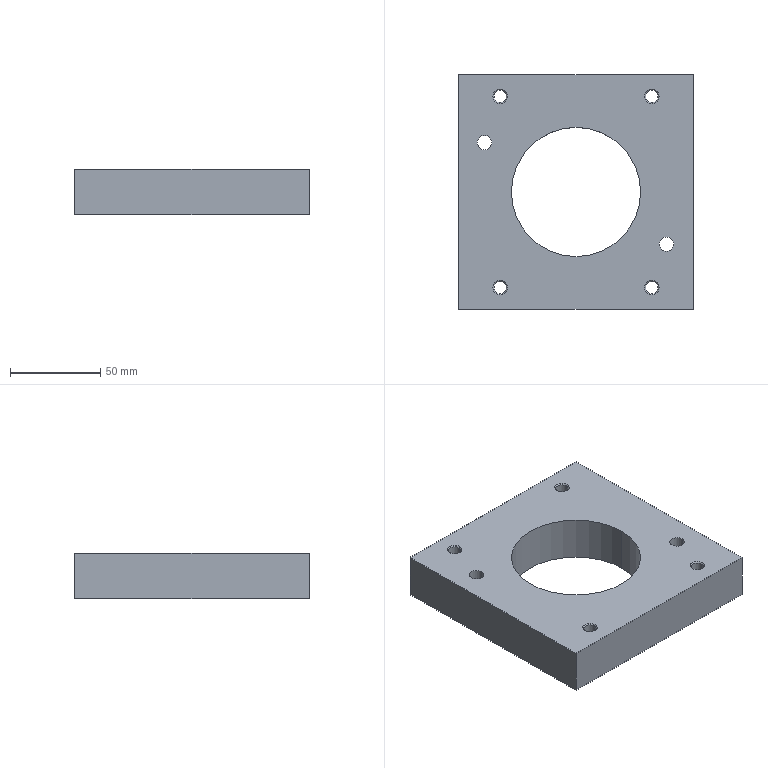Part | SolidWorks | features BaseBody 1 | 1 solid | 28 faces | box 130 x 130 x 25 mm | volume 315785 mm3 | cylinder 14 | cone 8 | plane 6 | commonest cylinder face diameters 6.806 x8 8 x4 71.56 x2
STEP:
#1=CARTESIAN_POINT('',(-131.403,-77.99,45.703));
#2=VERTEX_POINT('',#1);
#3=CARTESIAN_POINT('',(-124.597,-77.99,45.703));
#4=VERTEX_POINT('',#3);
#5=CARTESIAN_POINT('',(-128.,-77.99,45.703));
#6=DIRECTION('',(0.,0.,1.));
#7=DIRECTION('',(1.,0.,0.));
#8=AXIS2_PLACEMENT_3D('',#5,#6,#7);
#9=CIRCLE('',#8,3.403);
#10=EDGE_CURVE('',#2,#4,#9,.T.);
#11=ORIENTED_EDGE('',*,*,#10,.F.);
#12=CARTESIAN_POINT('',(-132.,-77.99,46.3));
#13=VERTEX_POINT('',#12);
#14=CARTESIAN_POINT('',(-132.,-77.99,46.3));
#15=DIRECTION('',(-0.7071,0.,0.7071));
#16=VECTOR('',#15,1000.);
#17=LINE('',#14,#16);
#18=EDGE_CURVE('',#2,#13,#17,.T.);
#19=ORIENTED_EDGE('',*,*,#18,.T.);
#20=CARTESIAN_POINT('',(-124.,-77.99,46.3));
#21=VERTEX_POINT('',#20);
#22=CARTESIAN_POINT('',(-128.,-77.99,46.3));
#23=DIRECTION('',(0.,0.,-1.));
#24=DIRECTION('',(0.7071,-0.7071,0.));
#25=AXIS2_PLACEMENT_3D('',#22,#23,#24);
#26=CIRCLE('',#25,4.);
#27=EDGE_CURVE('',#21,#13,#26,.T.);
#28=ORIENTED_EDGE('',*,*,#27,.F.);
#29=CARTESIAN_POINT('',(-124.,-77.99,46.3));
#30=DIRECTION('',(0.7071,0.,0.7071));
#31=VECTOR('',#30,1000.);
#32=LINE('',#29,#31);
#33=EDGE_CURVE('',#4,#21,#32,.T.);
#34=ORIENTED_EDGE('',*,*,#33,.F.);
#35=EDGE_LOOP('',(#11,#19,#28,#34));
#36=FACE_OUTER_BOUND('',#35,.T.);
#37=CARTESIAN_POINT('',(-128.,-77.99,46.3));
#38=DIRECTION('',(0.,0.,1.));
#39=DIRECTION('',(1.,0.,0.));
#40=AXIS2_PLACEMENT_3D('',#37,#38,#39);
#41=CONICAL_SURFACE('',#40,4.,0.7854);
#42=ADVANCED_FACE('',(#36),#41,.F.);
#43=CARTESIAN_POINT('',(-124.597,-77.99,21.3));
#44=VERTEX_POINT('',#43);
#45=CARTESIAN_POINT('',(-131.403,-77.99,21.3));
#46=VERTEX_POINT('',#45);
#47=CARTESIAN_POINT('',(-128.,-77.99,21.3));
#48=DIRECTION('',(0.,0.,-1.));
#49=DIRECTION('',(-1.,0.,0.));
#50=AXIS2_PLACEMENT_3D('',#47,#48,#49);
#51=CIRCLE('',#50,3.403);
#52=EDGE_CURVE('',#44,#46,#51,.T.);
#53=ORIENTED_EDGE('',*,*,#52,.T.);
#54=CARTESIAN_POINT('',(-131.403,-77.99,17.317));
#55=DIRECTION('',(0.,0.,1.));
#56=VECTOR('',#55,1000.);
#57=LINE('',#54,#56);
#58=EDGE_CURVE('',#46,#2,#57,.T.);
#59=ORIENTED_EDGE('',*,*,#58,.T.);
#60=ORIENTED_EDGE('',*,*,#10,.T.);
#61=CARTESIAN_POINT('',(-124.597,-77.99,17.317));
#62=DIRECTION('',(0.,0.,1.));
#63=VECTOR('',#62,1000.);
#64=LINE('',#61,#63);
#65=EDGE_CURVE('',#44,#4,#64,.T.);
#66=ORIENTED_EDGE('',*,*,#65,.F.);
#67=EDGE_LOOP('',(#53,#59,#60,#66));
#68=FACE_OUTER_BOUND('',#67,.T.);
#69=CARTESIAN_POINT('',(-128.,-77.99,17.317));
#70=DIRECTION('',(0.,0.,1.));
#71=DIRECTION('',(1.,0.,0.));
#72=AXIS2_PLACEMENT_3D('',#69,#70,#71);
#73=CYLINDRICAL_SURFACE('',#72,3.403);
#74=ADVANCED_FACE('',(#68),#73,.F.);
#75=CARTESIAN_POINT('',(-40.597,27.99,45.703));
#76=VERTEX_POINT('',#75);
#77=CARTESIAN_POINT('',(-47.403,27.99,45.703));
#78=VERTEX_POINT('',#77);
#79=CARTESIAN_POINT('',(-44.,27.99,45.703));
#80=DIRECTION('',(0.,0.,1.));
#81=DIRECTION('',(-1.,0.,0.));
#82=AXIS2_PLACEMENT_3D('',#79,#80,#81);
#83=CIRCLE('',#82,3.403);
#84=EDGE_CURVE('',#76,#78,#83,.T.);
#85=ORIENTED_EDGE('',*,*,#84,.F.);
#86=CARTESIAN_POINT('',(-40.,27.99,46.3));
#87=VERTEX_POINT('',#86);
#88=CARTESIAN_POINT('',(-40.,27.99,46.3));
#89=DIRECTION('',(0.7071,0.,0.7071));
#90=VECTOR('',#89,1000.);
#91=LINE('',#88,#90);
#92=EDGE_CURVE('',#76,#87,#91,.T.);
#93=ORIENTED_EDGE('',*,*,#92,.T.);
#94=CARTESIAN_POINT('',(-48.,27.99,46.3));
#95=VERTEX_POINT('',#94);
#96=CARTESIAN_POINT('',(-44.,27.99,46.3));
#97=DIRECTION('',(0.,0.,-1.));
#98=DIRECTION('',(-0.7071,0.7071,0.));
#99=AXIS2_PLACEMENT_3D('',#96,#97,#98);
#100=CIRCLE('',#99,4.);
#101=EDGE_CURVE('',#95,#87,#100,.T.);
#102=ORIENTED_EDGE('',*,*,#101,.F.);
#103=CARTESIAN_POINT('',(-48.,27.99,46.3));
#104=DIRECTION('',(-0.7071,0.,0.7071));
#105=VECTOR('',#104,1000.);
#106=LINE('',#103,#105);
#107=EDGE_CURVE('',#78,#95,#106,.T.);
#108=ORIENTED_EDGE('',*,*,#107,.F.);
#109=EDGE_LOOP('',(#85,#93,#102,#108));
#110=FACE_OUTER_BOUND('',#109,.T.);
#111=CARTESIAN_POINT('',(-44.,27.99,46.3));
#112=DIRECTION('',(0.,0.,1.));
#113=DIRECTION('',(-1.,0.,0.));
#114=AXIS2_PLACEMENT_3D('',#111,#112,#113);
#115=CONICAL_SURFACE('',#114,4.,0.7854);
#116=ADVANCED_FACE('',(#110),#115,.F.);
#117=CARTESIAN_POINT('',(-47.403,27.99,21.3));
#118=VERTEX_POINT('',#117);
#119=CARTESIAN_POINT('',(-40.597,27.99,21.3));
#120=VERTEX_POINT('',#119);
#121=CARTESIAN_POINT('',(-44.,27.99,21.3));
#122=DIRECTION('',(0.,0.,-1.));
#123=DIRECTION('',(-1.,0.,0.));
#124=AXIS2_PLACEMENT_3D('',#121,#122,#123);
#125=CIRCLE('',#124,3.403);
#126=EDGE_CURVE('',#118,#120,#125,.T.);
#127=ORIENTED_EDGE('',*,*,#126,.T.);
#128=CARTESIAN_POINT('',(-40.597,27.99,17.317));
#129=DIRECTION('',(0.,0.,1.));
#130=VECTOR('',#129,1000.);
#131=LINE('',#128,#130);
#132=EDGE_CURVE('',#120,#76,#131,.T.);
#133=ORIENTED_EDGE('',*,*,#132,.T.);
#134=ORIENTED_EDGE('',*,*,#84,.T.);
#135=CARTESIAN_POINT('',(-47.403,27.99,17.317));
#136=DIRECTION('',(0.,0.,1.));
#137=VECTOR('',#136,1000.);
#138=LINE('',#135,#137);
#139=EDGE_CURVE('',#118,#78,#138,.T.);
#140=ORIENTED_EDGE('',*,*,#139,.F.);
#141=EDGE_LOOP('',(#127,#133,#134,#140));
#142=FACE_OUTER_BOUND('',#141,.T.);
#143=CARTESIAN_POINT('',(-44.,27.99,17.317));
#144=DIRECTION('',(0.,0.,1.));
#145=DIRECTION('',(-1.,0.,0.));
#146=AXIS2_PLACEMENT_3D('',#143,#144,#145);
#147=CYLINDRICAL_SURFACE('',#146,3.403);
#148=ADVANCED_FACE('',(#142),#147,.F.);
#149=CARTESIAN_POINT('',(-140.678,2.312,21.3));
#150=VERTEX_POINT('',#149);
#151=CARTESIAN_POINT('',(-132.678,2.312,21.3));
#152=VERTEX_POINT('',#151);
#153=CARTESIAN_POINT('',(-136.678,2.312,21.3));
#154=DIRECTION('',(0.,0.,1.));
#155=DIRECTION('',(0.7071,0.7071,0.));
#156=AXIS2_PLACEMENT_3D('',#153,#154,#155);
#157=CIRCLE('',#156,4.);
#158=EDGE_CURVE('',#150,#152,#157,.T.);
#159=ORIENTED_EDGE('',*,*,#158,.F.);
#160=CARTESIAN_POINT('',(-140.678,2.312,46.3));
#161=VERTEX_POINT('',#160);
#162=CARTESIAN_POINT('',(-140.678,2.312,21.3));
#163=DIRECTION('',(0.,0.,1.));
#164=VECTOR('',#163,1000.);
#165=LINE('',#162,#164);
#166=EDGE_CURVE('',#150,#161,#165,.T.);
#167=ORIENTED_EDGE('',*,*,#166,.T.);
#168=CARTESIAN_POINT('',(-132.678,2.312,46.3));
#169=VERTEX_POINT('',#168);
#170=CARTESIAN_POINT('',(-136.678,2.312,46.3));
#171=DIRECTION('',(0.,0.,1.));
#172=DIRECTION('',(0.7071,0.7071,0.));
#173=AXIS2_PLACEMENT_3D('',#170,#171,#172);
#174=CIRCLE('',#173,4.);
#175=EDGE_CURVE('',#161,#169,#174,.T.);
#176=ORIENTED_EDGE('',*,*,#175,.T.);
#177=CARTESIAN_POINT('',(-132.678,2.312,21.3));
#178=DIRECTION('',(0.,0.,1.));
#179=VECTOR('',#178,1000.);
#180=LINE('',#177,#179);
#181=EDGE_CURVE('',#152,#169,#180,.T.);
#182=ORIENTED_EDGE('',*,*,#181,.F.);
#183=EDGE_LOOP('',(#159,#167,#176,#182));
#184=FACE_OUTER_BOUND('',#183,.T.);
#185=CARTESIAN_POINT('',(-136.678,2.312,21.3));
#186=DIRECTION('',(0.,0.,1.));
#187=DIRECTION('',(1.,0.,0.));
#188=AXIS2_PLACEMENT_3D('',#185,#186,#187);
#189=CYLINDRICAL_SURFACE('',#188,4.);
#190=ADVANCED_FACE('',(#184),#189,.F.);
#191=CARTESIAN_POINT('',(-39.858,-53.934,21.3));
#192=VERTEX_POINT('',#191);
#193=CARTESIAN_POINT('',(-31.858,-53.934,21.3));
#194=VERTEX_POINT('',#193);
#195=CARTESIAN_POINT('',(-35.858,-53.934,21.3));
#196=DIRECTION('',(0.,0.,1.));
#197=DIRECTION('',(0.7071,0.7071,0.));
#198=AXIS2_PLACEMENT_3D('',#195,#196,#197);
#199=CIRCLE('',#198,4.);
#200=EDGE_CURVE('',#192,#194,#199,.T.);
#201=ORIENTED_EDGE('',*,*,#200,.F.);
#202=CARTESIAN_POINT('',(-39.858,-53.934,46.3));
#203=VERTEX_POINT('',#202);
#204=CARTESIAN_POINT('',(-39.858,-53.934,21.3));
#205=DIRECTION('',(0.,0.,1.));
#206=VECTOR('',#205,1000.);
#207=LINE('',#204,#206);
#208=EDGE_CURVE('',#192,#203,#207,.T.);
#209=ORIENTED_EDGE('',*,*,#208,.T.);
#210=CARTESIAN_POINT('',(-31.858,-53.934,46.3));
#211=VERTEX_POINT('',#210);
#212=CARTESIAN_POINT('',(-35.858,-53.934,46.3));
#213=DIRECTION('',(0.,0.,1.));
#214=DIRECTION('',(0.7071,0.7071,0.));
#215=AXIS2_PLACEMENT_3D('',#212,#213,#214);
#216=CIRCLE('',#215,4.);
#217=EDGE_CURVE('',#203,#211,#216,.T.);
#218=ORIENTED_EDGE('',*,*,#217,.T.);
#219=CARTESIAN_POINT('',(-31.858,-53.934,21.3));
#220=DIRECTION('',(0.,0.,1.));
#221=VECTOR('',#220,1000.);
#222=LINE('',#219,#221);
#223=EDGE_CURVE('',#194,#211,#222,.T.);
#224=ORIENTED_EDGE('',*,*,#223,.F.);
#225=EDGE_LOOP('',(#201,#209,#218,#224));
#226=FACE_OUTER_BOUND('',#225,.T.);
#227=CARTESIAN_POINT('',(-35.858,-53.934,21.3));
#228=DIRECTION('',(0.,0.,1.));
#229=DIRECTION('',(1.,0.,0.));
#230=AXIS2_PLACEMENT_3D('',#227,#228,#229);
#231=CYLINDRICAL_SURFACE('',#230,4.);
#232=ADVANCED_FACE('',(#226),#231,.F.);
#233=CARTESIAN_POINT('',(-47.403,-77.99,45.703));
#234=VERTEX_POINT('',#233);
#235=CARTESIAN_POINT('',(-40.597,-77.99,45.703));
#236=VERTEX_POINT('',#235);
#237=CARTESIAN_POINT('',(-44.,-77.99,45.703));
#238=DIRECTION('',(0.,0.,-1.));
#239=DIRECTION('',(-1.,0.,0.));
#240=AXIS2_PLACEMENT_3D('',#237,#238,#239);
#241=CIRCLE('',#240,3.403);
#242=EDGE_CURVE('',#234,#236,#241,.T.);
#243=ORIENTED_EDGE('',*,*,#242,.T.);
#244=CARTESIAN_POINT('',(-40.,-77.99,46.3));
#245=VERTEX_POINT('',#244);
#246=CARTESIAN_POINT('',(-40.,-77.99,46.3));
#247=DIRECTION('',(0.7071,0.,0.7071));
#248=VECTOR('',#247,1000.);
#249=LINE('',#246,#248);
#250=EDGE_CURVE('',#236,#245,#249,.T.);
#251=ORIENTED_EDGE('',*,*,#250,.T.);
#252=CARTESIAN_POINT('',(-48.,-77.99,46.3));
#253=VERTEX_POINT('',#252);
#254=CARTESIAN_POINT('',(-44.,-77.99,46.3));
#255=DIRECTION('',(0.,0.,1.));
#256=DIRECTION('',(-0.7071,-0.7071,0.));
#257=AXIS2_PLACEMENT_3D('',#254,#255,#256);
#258=CIRCLE('',#257,4.);
#259=EDGE_CURVE('',#245,#253,#258,.T.);
#260=ORIENTED_EDGE('',*,*,#259,.T.);
#261=CARTESIAN_POINT('',(-48.,-77.99,46.3));
#262=DIRECTION('',(-0.7071,0.,0.7071));
#263=VECTOR('',#262,1000.);
#264=LINE('',#261,#263);
#265=EDGE_CURVE('',#234,#253,#264,.T.);
#266=ORIENTED_EDGE('',*,*,#265,.F.);
#267=EDGE_LOOP('',(#243,#251,#260,#266));
#268=FACE_OUTER_BOUND('',#267,.T.);
#269=CARTESIAN_POINT('',(-44.,-77.99,46.3));
#270=DIRECTION('',(0.,0.,1.));
#271=DIRECTION('',(-1.,0.,0.));
#272=AXIS2_PLACEMENT_3D('',#269,#270,#271);
#273=CONICAL_SURFACE('',#272,4.,0.7854);
#274=ADVANCED_FACE('',(#268),#273,.F.);
#275=CARTESIAN_POINT('',(-47.403,-77.99,21.3));
#276=VERTEX_POINT('',#275);
#277=CARTESIAN_POINT('',(-40.597,-77.99,21.3));
#278=VERTEX_POINT('',#277);
#279=CARTESIAN_POINT('',(-44.,-77.99,21.3));
#280=DIRECTION('',(0.,0.,-1.));
#281=DIRECTION('',(-1.,0.,0.));
#282=AXIS2_PLACEMENT_3D('',#279,#280,#281);
#283=CIRCLE('',#282,3.403);
#284=EDGE_CURVE('',#276,#278,#283,.T.);
#285=ORIENTED_EDGE('',*,*,#284,.T.);
#286=CARTESIAN_POINT('',(-40.597,-77.99,17.317));
#287=DIRECTION('',(0.,0.,1.));
#288=VECTOR('',#287,1000.);
#289=LINE('',#286,#288);
#290=EDGE_CURVE('',#278,#236,#289,.T.);
#291=ORIENTED_EDGE('',*,*,#290,.T.);
#292=ORIENTED_EDGE('',*,*,#242,.F.);
#293=CARTESIAN_POINT('',(-47.403,-77.99,17.317));
#294=DIRECTION('',(0.,0.,1.));
#295=VECTOR('',#294,1000.);
#296=LINE('',#293,#295);
#297=EDGE_CURVE('',#276,#234,#296,.T.);
#298=ORIENTED_EDGE('',*,*,#297,.F.);
#299=EDGE_LOOP('',(#285,#291,#292,#298));
#300=FACE_OUTER_BOUND('',#299,.T.);
#301=CARTESIAN_POINT('',(-44.,-77.99,17.317));
#302=DIRECTION('',(0.,0.,1.));
#303=DIRECTION('',(-1.,0.,0.));
#304=AXIS2_PLACEMENT_3D('',#301,#302,#303);
#305=CYLINDRICAL_SURFACE('',#304,3.403);
#306=ADVANCED_FACE('',(#300),#305,.F.);
#307=CARTESIAN_POINT('',(-124.597,27.99,45.703));
#308=VERTEX_POINT('',#307);
#309=CARTESIAN_POINT('',(-131.403,27.99,45.703));
#310=VERTEX_POINT('',#309);
#311=CARTESIAN_POINT('',(-128.,27.99,45.703));
#312=DIRECTION('',(0.,0.,-1.));
#313=DIRECTION('',(1.,0.,0.));
#314=AXIS2_PLACEMENT_3D('',#311,#312,#313);
#315=CIRCLE('',#314,3.403);
#316=EDGE_CURVE('',#308,#310,#315,.T.);
#317=ORIENTED_EDGE('',*,*,#316,.T.);
#318=CARTESIAN_POINT('',(-132.,27.99,46.3));
#319=VERTEX_POINT('',#318);
#320=CARTESIAN_POINT('',(-132.,27.99,46.3));
#321=DIRECTION('',(-0.7071,0.,0.7071));
#322=VECTOR('',#321,1000.);
#323=LINE('',#320,#322);
#324=EDGE_CURVE('',#310,#319,#323,.T.);
#325=ORIENTED_EDGE('',*,*,#324,.T.);
#326=CARTESIAN_POINT('',(-124.,27.99,46.3));
#327=VERTEX_POINT('',#326);
#328=CARTESIAN_POINT('',(-128.,27.99,46.3));
#329=DIRECTION('',(0.,0.,1.));
#330=DIRECTION('',(0.7071,0.7071,0.));
#331=AXIS2_PLACEMENT_3D('',#328,#329,#330);
#332=CIRCLE('',#331,4.);
#333=EDGE_CURVE('',#319,#327,#332,.T.);
#334=ORIENTED_EDGE('',*,*,#333,.T.);
#335=CARTESIAN_POINT('',(-124.,27.99,46.3));
#336=DIRECTION('',(0.7071,0.,0.7071));
#337=VECTOR('',#336,1000.);
#338=LINE('',#335,#337);
#339=EDGE_CURVE('',#308,#327,#338,.T.);
#340=ORIENTED_EDGE('',*,*,#339,.F.);
#341=EDGE_LOOP('',(#317,#325,#334,#340));
#342=FACE_OUTER_BOUND('',#341,.T.);
#343=CARTESIAN_POINT('',(-128.,27.99,46.3));
#344=DIRECTION('',(0.,0.,1.));
#345=DIRECTION('',(1.,0.,0.));
#346=AXIS2_PLACEMENT_3D('',#343,#344,#345);
#347=CONICAL_SURFACE('',#346,4.,0.7854);
#348=ADVANCED_FACE('',(#342),#347,.F.);
#349=CARTESIAN_POINT('',(-124.597,27.99,21.3));
#350=VERTEX_POINT('',#349);
#351=CARTESIAN_POINT('',(-131.403,27.99,21.3));
#352=VERTEX_POINT('',#351);
#353=CARTESIAN_POINT('',(-128.,27.99,21.3));
#354=DIRECTION('',(0.,0.,-1.));
#355=DIRECTION('',(-1.,0.,0.));
#356=AXIS2_PLACEMENT_3D('',#353,#354,#355);
#357=CIRCLE('',#356,3.403);
#358=EDGE_CURVE('',#350,#352,#357,.T.);
#359=ORIENTED_EDGE('',*,*,#358,.T.);
#360=CARTESIAN_POINT('',(-131.403,27.99,17.317));
#361=DIRECTION('',(0.,0.,1.));
#362=VECTOR('',#361,1000.);
#363=LINE('',#360,#362);
#364=EDGE_CURVE('',#352,#310,#363,.T.);
#365=ORIENTED_EDGE('',*,*,#364,.T.);
#366=ORIENTED_EDGE('',*,*,#316,.F.);
#367=CARTESIAN_POINT('',(-124.597,27.99,17.317));
#368=DIRECTION('',(0.,0.,1.));
#369=VECTOR('',#368,1000.);
#370=LINE('',#367,#369);
#371=EDGE_CURVE('',#350,#308,#370,.T.);
#372=ORIENTED_EDGE('',*,*,#371,.F.);
#373=EDGE_LOOP('',(#359,#365,#366,#372));
#374=FACE_OUTER_BOUND('',#373,.T.);
#375=CARTESIAN_POINT('',(-128.,27.99,17.317));
#376=DIRECTION('',(0.,0.,1.));
#377=DIRECTION('',(1.,0.,0.));
#378=AXIS2_PLACEMENT_3D('',#375,#376,#377);
#379=CYLINDRICAL_SURFACE('',#378,3.403);
#380=ADVANCED_FACE('',(#374),#379,.F.);
#381=CARTESIAN_POINT('',(-50.22,-25.,46.3));
#382=VERTEX_POINT('',#381);
#383=CARTESIAN_POINT('',(-121.78,-25.,46.3));
#384=VERTEX_POINT('',#383);
#385=CARTESIAN_POINT('',(-86.,-25.,46.3));
#386=DIRECTION('',(0.,0.,-1.));
#387=DIRECTION('',(-1.,0.,0.));
#388=AXIS2_PLACEMENT_3D('',#385,#386,#387);
#389=CIRCLE('',#388,35.78);
#390=EDGE_CURVE('',#382,#384,#389,.T.);
#391=ORIENTED_EDGE('',*,*,#390,.F.);
#392=CARTESIAN_POINT('',(-50.22,-25.,21.3));
#393=VERTEX_POINT('',#392);
#394=CARTESIAN_POINT('',(-50.22,-25.,21.3));
#395=DIRECTION('',(0.,0.,-1.));
#396=VECTOR('',#395,1000.);
#397=LINE('',#394,#396);
#398=EDGE_CURVE('',#382,#393,#397,.T.);
#399=ORIENTED_EDGE('',*,*,#398,.T.);
#400=CARTESIAN_POINT('',(-121.78,-25.,21.3));
#401=VERTEX_POINT('',#400);
#402=CARTESIAN_POINT('',(-86.,-25.,21.3));
#403=DIRECTION('',(0.,0.,-1.));
#404=DIRECTION('',(-1.,0.,0.));
#405=AXIS2_PLACEMENT_3D('',#402,#403,#404);
#406=CIRCLE('',#405,35.78);
#407=EDGE_CURVE('',#393,#401,#406,.T.);
#408=ORIENTED_EDGE('',*,*,#407,.T.);
#409=CARTESIAN_POINT('',(-121.78,-25.,21.3));
#410=DIRECTION('',(0.,0.,-1.));
#411=VECTOR('',#410,1000.);
#412=LINE('',#409,#411);
#413=EDGE_CURVE('',#384,#401,#412,.T.);
#414=ORIENTED_EDGE('',*,*,#413,.F.);
#415=EDGE_LOOP('',(#391,#399,#408,#414));
#416=FACE_OUTER_BOUND('',#415,.T.);
#417=CARTESIAN_POINT('',(-86.,-25.,21.3));
#418=DIRECTION('',(0.,0.,-1.));
#419=DIRECTION('',(-1.,0.,0.));
#420=AXIS2_PLACEMENT_3D('',#417,#418,#419);
#421=CYLINDRICAL_SURFACE('',#420,35.78);
#422=ADVANCED_FACE('',(#416),#421,.F.);
#423=CARTESIAN_POINT('',(-21.,40.,21.3));
#424=VERTEX_POINT('',#423);
#425=CARTESIAN_POINT('',(-21.,40.,46.3));
#426=VERTEX_POINT('',#425);
#427=CARTESIAN_POINT('',(-21.,40.,21.3));
#428=DIRECTION('',(0.,0.,1.));
#429=VECTOR('',#428,1000.);
#430=LINE('',#427,#429);
#431=EDGE_CURVE('',#424,#426,#430,.T.);
#432=ORIENTED_EDGE('',*,*,#431,.F.);
#433=CARTESIAN_POINT('',(-151.,40.,21.3));
#434=VERTEX_POINT('',#433);
#435=CARTESIAN_POINT('',(-86.,40.,21.3));
#436=DIRECTION('',(-1.,0.,0.));
#437=VECTOR('',#436,1000.);
#438=LINE('',#435,#437);
#439=EDGE_CURVE('',#424,#434,#438,.T.);
#440=ORIENTED_EDGE('',*,*,#439,.T.);
#441=CARTESIAN_POINT('',(-151.,40.,46.3));
#442=VERTEX_POINT('',#441);
#443=CARTESIAN_POINT('',(-151.,40.,21.3));
#444=DIRECTION('',(0.,0.,1.));
#445=VECTOR('',#444,1000.);
#446=LINE('',#443,#445);
#447=EDGE_CURVE('',#434,#442,#446,.T.);
#448=ORIENTED_EDGE('',*,*,#447,.T.);
#449=CARTESIAN_POINT('',(-86.,40.,46.3));
#450=DIRECTION('',(-1.,0.,0.));
#451=VECTOR('',#450,1000.);
#452=LINE('',#449,#451);
#453=EDGE_CURVE('',#426,#442,#452,.T.);
#454=ORIENTED_EDGE('',*,*,#453,.F.);
#455=EDGE_LOOP('',(#432,#440,#448,#454));
#456=FACE_OUTER_BOUND('',#455,.T.);
#457=CARTESIAN_POINT('',(-86.,40.,21.3));
#458=DIRECTION('',(0.,-1.,0.));
#459=DIRECTION('',(-1.,0.,0.));
#460=AXIS2_PLACEMENT_3D('',#457,#458,#459);
#461=PLANE('',#460);
#462=ADVANCED_FACE('',(#456),#461,.F.);
#463=ORIENTED_EDGE('',*,*,#447,.F.);
#464=CARTESIAN_POINT('',(-151.,-90.,21.3));
#465=VERTEX_POINT('',#464);
#466=CARTESIAN_POINT('',(-151.,-25.,21.3));
#467=DIRECTION('',(0.,-1.,0.));
#468=VECTOR('',#467,1000.);
#469=LINE('',#466,#468);
#470=EDGE_CURVE('',#434,#465,#469,.T.);
#471=ORIENTED_EDGE('',*,*,#470,.T.);
#472=CARTESIAN_POINT('',(-151.,-90.,46.3));
#473=VERTEX_POINT('',#472);
#474=CARTESIAN_POINT('',(-151.,-90.,21.3));
#475=DIRECTION('',(0.,0.,1.));
#476=VECTOR('',#475,1000.);
#477=LINE('',#474,#476);
#478=EDGE_CURVE('',#465,#473,#477,.T.);
#479=ORIENTED_EDGE('',*,*,#478,.T.);
#480=CARTESIAN_POINT('',(-151.,-25.,46.3));
#481=DIRECTION('',(0.,-1.,0.));
#482=VECTOR('',#481,1000.);
#483=LINE('',#480,#482);
#484=EDGE_CURVE('',#442,#473,#483,.T.);
#485=ORIENTED_EDGE('',*,*,#484,.F.);
#486=EDGE_LOOP('',(#463,#471,#479,#485));
#487=FACE_OUTER_BOUND('',#486,.T.);
#488=CARTESIAN_POINT('',(-151.,-25.,21.3));
#489=DIRECTION('',(1.,0.,0.));
#490=DIRECTION('',(0.,-1.,0.));
#491=AXIS2_PLACEMENT_3D('',#488,#489,#490);
#492=PLANE('',#491);
#493=ADVANCED_FACE('',(#487),#492,.F.);
#494=ORIENTED_EDGE('',*,*,#478,.F.);
#495=CARTESIAN_POINT('',(-21.,-90.,21.3));
#496=VERTEX_POINT('',#495);
#497=CARTESIAN_POINT('',(-86.,-90.,21.3));
#498=DIRECTION('',(1.,0.,0.));
#499=VECTOR('',#498,1000.);
#500=LINE('',#497,#499);
#501=EDGE_CURVE('',#465,#496,#500,.T.);
#502=ORIENTED_EDGE('',*,*,#501,.T.);
#503=CARTESIAN_POINT('',(-21.,-90.,46.3));
#504=VERTEX_POINT('',#503);
#505=CARTESIAN_POINT('',(-21.,-90.,21.3));
#506=DIRECTION('',(0.,0.,1.));
#507=VECTOR('',#506,1000.);
#508=LINE('',#505,#507);
#509=EDGE_CURVE('',#496,#504,#508,.T.);
#510=ORIENTED_EDGE('',*,*,#509,.T.);
#511=CARTESIAN_POINT('',(-86.,-90.,46.3));
#512=DIRECTION('',(1.,0.,0.));
#513=VECTOR('',#512,1000.);
#514=LINE('',#511,#513);
#515=EDGE_CURVE('',#473,#504,#514,.T.);
#516=ORIENTED_EDGE('',*,*,#515,.F.);
#517=EDGE_LOOP('',(#494,#502,#510,#516));
#518=FACE_OUTER_BOUND('',#517,.T.);
#519=CARTESIAN_POINT('',(-86.,-90.,21.3));
#520=DIRECTION('',(0.,1.,0.));
#521=DIRECTION('',(1.,0.,0.));
#522=AXIS2_PLACEMENT_3D('',#519,#520,#521);
#523=PLANE('',#522);
#524=ADVANCED_FACE('',(#518),#523,.F.);
#525=ORIENTED_EDGE('',*,*,#398,.F.);
#526=CARTESIAN_POINT('',(-86.,-25.,46.3));
#527=DIRECTION('',(0.,0.,-1.));
#528=DIRECTION('',(-1.,0.,0.));
#529=AXIS2_PLACEMENT_3D('',#526,#527,#528);
#530=CIRCLE('',#529,35.78);
#531=EDGE_CURVE('',#384,#382,#530,.T.);
#532=ORIENTED_EDGE('',*,*,#531,.F.);
#533=ORIENTED_EDGE('',*,*,#413,.T.);
#534=CARTESIAN_POINT('',(-86.,-25.,21.3));
#535=DIRECTION('',(0.,0.,-1.));
#536=DIRECTION('',(-1.,0.,0.));
#537=AXIS2_PLACEMENT_3D('',#534,#535,#536);
#538=CIRCLE('',#537,35.78);
#539=EDGE_CURVE('',#401,#393,#538,.T.);
#540=ORIENTED_EDGE('',*,*,#539,.T.);
#541=EDGE_LOOP('',(#525,#532,#533,#540));
#542=FACE_OUTER_BOUND('',#541,.T.);
#543=CARTESIAN_POINT('',(-86.,-25.,21.3));
#544=DIRECTION('',(0.,0.,-1.));
#545=DIRECTION('',(-1.,0.,0.));
#546=AXIS2_PLACEMENT_3D('',#543,#544,#545);
#547=CYLINDRICAL_SURFACE('',#546,35.78);
#548=ADVANCED_FACE('',(#542),#547,.F.);
#549=CARTESIAN_POINT('',(-21.,-25.,21.3));
#550=DIRECTION('',(0.,1.,0.));
#551=VECTOR('',#550,1000.);
#552=LINE('',#549,#551);
#553=EDGE_CURVE('',#496,#424,#552,.T.);
#554=ORIENTED_EDGE('',*,*,#553,.T.);
#555=ORIENTED_EDGE('',*,*,#431,.T.);
#556=CARTESIAN_POINT('',(-21.,-25.,46.3));
#557=DIRECTION('',(0.,1.,0.));
#558=VECTOR('',#557,1000.);
#559=LINE('',#556,#558);
#560=EDGE_CURVE('',#504,#426,#559,.T.);
#561=ORIENTED_EDGE('',*,*,#560,.F.);
#562=ORIENTED_EDGE('',*,*,#509,.F.);
#563=EDGE_LOOP('',(#554,#555,#561,#562));
#564=FACE_OUTER_BOUND('',#563,.T.);
#565=CARTESIAN_POINT('',(-21.,-25.,21.3));
#566=DIRECTION('',(-1.,0.,0.));
#567=DIRECTION('',(0.,1.,0.));
#568=AXIS2_PLACEMENT_3D('',#565,#566,#567);
#569=PLANE('',#568);
#570=ADVANCED_FACE('',(#564),#569,.F.);
#571=ORIENTED_EDGE('',*,*,#27,.T.);
#572=CARTESIAN_POINT('',(-128.,-77.99,46.3));
#573=DIRECTION('',(0.,0.,-1.));
#574=DIRECTION('',(0.7071,-0.7071,0.));
#575=AXIS2_PLACEMENT_3D('',#572,#573,#574);
#576=CIRCLE('',#575,4.);
#577=EDGE_CURVE('',#13,#21,#576,.T.);
#578=ORIENTED_EDGE('',*,*,#577,.T.);
#579=EDGE_LOOP('',(#571,#578));
#580=FACE_BOUND('',#579,.T.);
#581=ORIENTED_EDGE('',*,*,#101,.T.);
#582=CARTESIAN_POINT('',(-44.,27.99,46.3));
#583=DIRECTION('',(0.,0.,-1.));
#584=DIRECTION('',(-0.7071,0.7071,0.));
#585=AXIS2_PLACEMENT_3D('',#582,#583,#584);
#586=CIRCLE('',#585,4.);
#587=EDGE_CURVE('',#87,#95,#586,.T.);
#588=ORIENTED_EDGE('',*,*,#587,.T.);
#589=EDGE_LOOP('',(#581,#588));
#590=FACE_BOUND('',#589,.T.);
#591=CARTESIAN_POINT('',(-136.678,2.312,46.3));
#592=DIRECTION('',(0.,0.,1.));
#593=DIRECTION('',(0.7071,0.7071,0.));
#594=AXIS2_PLACEMENT_3D('',#591,#592,#593);
#595=CIRCLE('',#594,4.);
#596=EDGE_CURVE('',#169,#161,#595,.T.);
#597=ORIENTED_EDGE('',*,*,#596,.F.);
#598=ORIENTED_EDGE('',*,*,#175,.F.);
#599=EDGE_LOOP('',(#597,#598));
#600=FACE_BOUND('',#599,.T.);
#601=CARTESIAN_POINT('',(-35.858,-53.934,46.3));
#602=DIRECTION('',(0.,0.,1.));
#603=DIRECTION('',(0.7071,0.7071,0.));
#604=AXIS2_PLACEMENT_3D('',#601,#602,#603);
#605=CIRCLE('',#604,4.);
#606=EDGE_CURVE('',#211,#203,#605,.T.);
#607=ORIENTED_EDGE('',*,*,#606,.F.);
#608=ORIENTED_EDGE('',*,*,#217,.F.);
#609=EDGE_LOOP('',(#607,#608));
#610=FACE_BOUND('',#609,.T.);
#611=CARTESIAN_POINT('',(-44.,-77.99,46.3));
#612=DIRECTION('',(0.,0.,1.));
#613=DIRECTION('',(-0.7071,-0.7071,0.));
#614=AXIS2_PLACEMENT_3D('',#611,#612,#613);
#615=CIRCLE('',#614,4.);
#616=EDGE_CURVE('',#253,#245,#615,.T.);
#617=ORIENTED_EDGE('',*,*,#616,.F.);
#618=ORIENTED_EDGE('',*,*,#259,.F.);
#619=EDGE_LOOP('',(#617,#618));
#620=FACE_BOUND('',#619,.T.);
#621=CARTESIAN_POINT('',(-128.,27.99,46.3));
#622=DIRECTION('',(0.,0.,1.));
#623=DIRECTION('',(0.7071,0.7071,0.));
#624=AXIS2_PLACEMENT_3D('',#621,#622,#623);
#625=CIRCLE('',#624,4.);
#626=EDGE_CURVE('',#327,#319,#625,.T.);
#627=ORIENTED_EDGE('',*,*,#626,.F.);
#628=ORIENTED_EDGE('',*,*,#333,.F.);
#629=EDGE_LOOP('',(#627,#628));
#630=FACE_BOUND('',#629,.T.);
#631=ORIENTED_EDGE('',*,*,#531,.T.);
#632=ORIENTED_EDGE('',*,*,#390,.T.);
#633=EDGE_LOOP('',(#631,#632));
#634=FACE_BOUND('',#633,.T.);
#635=ORIENTED_EDGE('',*,*,#515,.T.);
#636=ORIENTED_EDGE('',*,*,#560,.T.);
#637=ORIENTED_EDGE('',*,*,#453,.T.);
#638=ORIENTED_EDGE('',*,*,#484,.T.);
#639=EDGE_LOOP('',(#635,#636,#637,#638));
#640=FACE_OUTER_BOUND('',#639,.T.);
#641=CARTESIAN_POINT('',(-86.,-25.,46.3));
#642=DIRECTION('',(0.,0.,-1.));
#643=DIRECTION('',(-1.,0.,0.));
#644=AXIS2_PLACEMENT_3D('',#641,#642,#643);
#645=PLANE('',#644);
#646=ADVANCED_FACE('',(#580,#590,#600,#610,#620,#630,#634,#640),#645,.F.);
#647=ORIENTED_EDGE('',*,*,#52,.F.);
#648=CARTESIAN_POINT('',(-128.,-77.99,21.3));
#649=DIRECTION('',(0.,0.,-1.));
#650=DIRECTION('',(-1.,0.,0.));
#651=AXIS2_PLACEMENT_3D('',#648,#649,#650);
#652=CIRCLE('',#651,3.403);
#653=EDGE_CURVE('',#46,#44,#652,.T.);
#654=ORIENTED_EDGE('',*,*,#653,.F.);
#655=EDGE_LOOP('',(#647,#654));
#656=FACE_BOUND('',#655,.T.);
#657=ORIENTED_EDGE('',*,*,#126,.F.);
#658=CARTESIAN_POINT('',(-44.,27.99,21.3));
#659=DIRECTION('',(0.,0.,-1.));
#660=DIRECTION('',(-1.,0.,0.));
#661=AXIS2_PLACEMENT_3D('',#658,#659,#660);
#662=CIRCLE('',#661,3.403);
#663=EDGE_CURVE('',#120,#118,#662,.T.);
#664=ORIENTED_EDGE('',*,*,#663,.F.);
#665=EDGE_LOOP('',(#657,#664));
#666=FACE_BOUND('',#665,.T.);
#667=CARTESIAN_POINT('',(-136.678,2.312,21.3));
#668=DIRECTION('',(0.,0.,1.));
#669=DIRECTION('',(0.7071,0.7071,0.));
#670=AXIS2_PLACEMENT_3D('',#667,#668,#669);
#671=CIRCLE('',#670,4.);
#672=EDGE_CURVE('',#152,#150,#671,.T.);
#673=ORIENTED_EDGE('',*,*,#672,.T.);
#674=ORIENTED_EDGE('',*,*,#158,.T.);
#675=EDGE_LOOP('',(#673,#674));
#676=FACE_BOUND('',#675,.T.);
#677=CARTESIAN_POINT('',(-35.858,-53.934,21.3));
#678=DIRECTION('',(0.,0.,1.));
#679=DIRECTION('',(0.7071,0.7071,0.));
#680=AXIS2_PLACEMENT_3D('',#677,#678,#679);
#681=CIRCLE('',#680,4.);
#682=EDGE_CURVE('',#194,#192,#681,.T.);
#683=ORIENTED_EDGE('',*,*,#682,.T.);
#684=ORIENTED_EDGE('',*,*,#200,.T.);
#685=EDGE_LOOP('',(#683,#684));
#686=FACE_BOUND('',#685,.T.);
#687=ORIENTED_EDGE('',*,*,#284,.F.);
#688=CARTESIAN_POINT('',(-44.,-77.99,21.3));
#689=DIRECTION('',(0.,0.,-1.));
#690=DIRECTION('',(-1.,0.,0.));
#691=AXIS2_PLACEMENT_3D('',#688,#689,#690);
#692=CIRCLE('',#691,3.403);
#693=EDGE_CURVE('',#278,#276,#692,.T.);
#694=ORIENTED_EDGE('',*,*,#693,.F.);
#695=EDGE_LOOP('',(#687,#694));
#696=FACE_BOUND('',#695,.T.);
#697=ORIENTED_EDGE('',*,*,#358,.F.);
#698=CARTESIAN_POINT('',(-128.,27.99,21.3));
#699=DIRECTION('',(0.,0.,-1.));
#700=DIRECTION('',(-1.,0.,0.));
#701=AXIS2_PLACEMENT_3D('',#698,#699,#700);
#702=CIRCLE('',#701,3.403);
#703=EDGE_CURVE('',#352,#350,#702,.T.);
#704=ORIENTED_EDGE('',*,*,#703,.F.);
#705=EDGE_LOOP('',(#697,#704));
#706=FACE_BOUND('',#705,.T.);
#707=ORIENTED_EDGE('',*,*,#539,.F.);
#708=ORIENTED_EDGE('',*,*,#407,.F.);
#709=EDGE_LOOP('',(#707,#708));
#710=FACE_BOUND('',#709,.T.);
#711=ORIENTED_EDGE('',*,*,#501,.F.);
#712=ORIENTED_EDGE('',*,*,#470,.F.);
#713=ORIENTED_EDGE('',*,*,#439,.F.);
#714=ORIENTED_EDGE('',*,*,#553,.F.);
#715=EDGE_LOOP('',(#711,#712,#713,#714));
#716=FACE_OUTER_BOUND('',#715,.T.);
#717=CARTESIAN_POINT('',(-86.,-25.,21.3));
#718=DIRECTION('',(0.,0.,-1.));
#719=DIRECTION('',(-1.,0.,0.));
#720=AXIS2_PLACEMENT_3D('',#717,#718,#719);
#721=PLANE('',#720);
#722=ADVANCED_FACE('',(#656,#666,#676,#686,#696,#706,#710,#716),#721,.T.);
#723=ORIENTED_EDGE('',*,*,#364,.F.);
#724=ORIENTED_EDGE('',*,*,#703,.T.);
#725=ORIENTED_EDGE('',*,*,#371,.T.);
#726=CARTESIAN_POINT('',(-128.,27.99,45.703));
#727=DIRECTION('',(0.,0.,-1.));
#728=DIRECTION('',(1.,0.,0.));
#729=AXIS2_PLACEMENT_3D('',#726,#727,#728);
#730=CIRCLE('',#729,3.403);
#731=EDGE_CURVE('',#310,#308,#730,.T.);
#732=ORIENTED_EDGE('',*,*,#731,.F.);
#733=EDGE_LOOP('',(#723,#724,#725,#732));
#734=FACE_OUTER_BOUND('',#733,.T.);
#735=CARTESIAN_POINT('',(-128.,27.99,17.317));
#736=DIRECTION('',(0.,0.,1.));
#737=DIRECTION('',(1.,0.,0.));
#738=AXIS2_PLACEMENT_3D('',#735,#736,#737);
#739=CYLINDRICAL_SURFACE('',#738,3.403);
#740=ADVANCED_FACE('',(#734),#739,.F.);
#741=ORIENTED_EDGE('',*,*,#324,.F.);
#742=ORIENTED_EDGE('',*,*,#731,.T.);
#743=ORIENTED_EDGE('',*,*,#339,.T.);
#744=ORIENTED_EDGE('',*,*,#626,.T.);
#745=EDGE_LOOP('',(#741,#742,#743,#744));
#746=FACE_OUTER_BOUND('',#745,.T.);
#747=CARTESIAN_POINT('',(-128.,27.99,46.3));
#748=DIRECTION('',(0.,0.,1.));
#749=DIRECTION('',(1.,0.,0.));
#750=AXIS2_PLACEMENT_3D('',#747,#748,#749);
#751=CONICAL_SURFACE('',#750,4.,0.7854);
#752=ADVANCED_FACE('',(#746),#751,.F.);
#753=ORIENTED_EDGE('',*,*,#290,.F.);
#754=ORIENTED_EDGE('',*,*,#693,.T.);
#755=ORIENTED_EDGE('',*,*,#297,.T.);
#756=CARTESIAN_POINT('',(-44.,-77.99,45.703));
#757=DIRECTION('',(0.,0.,-1.));
#758=DIRECTION('',(-1.,0.,0.));
#759=AXIS2_PLACEMENT_3D('',#756,#757,#758);
#760=CIRCLE('',#759,3.403);
#761=EDGE_CURVE('',#236,#234,#760,.T.);
#762=ORIENTED_EDGE('',*,*,#761,.F.);
#763=EDGE_LOOP('',(#753,#754,#755,#762));
#764=FACE_OUTER_BOUND('',#763,.T.);
#765=CARTESIAN_POINT('',(-44.,-77.99,17.317));
#766=DIRECTION('',(0.,0.,1.));
#767=DIRECTION('',(-1.,0.,0.));
#768=AXIS2_PLACEMENT_3D('',#765,#766,#767);
#769=CYLINDRICAL_SURFACE('',#768,3.403);
#770=ADVANCED_FACE('',(#764),#769,.F.);
#771=ORIENTED_EDGE('',*,*,#250,.F.);
#772=ORIENTED_EDGE('',*,*,#761,.T.);
#773=ORIENTED_EDGE('',*,*,#265,.T.);
#774=ORIENTED_EDGE('',*,*,#616,.T.);
#775=EDGE_LOOP('',(#771,#772,#773,#774));
#776=FACE_OUTER_BOUND('',#775,.T.);
#777=CARTESIAN_POINT('',(-44.,-77.99,46.3));
#778=DIRECTION('',(0.,0.,1.));
#779=DIRECTION('',(-1.,0.,0.));
#780=AXIS2_PLACEMENT_3D('',#777,#778,#779);
#781=CONICAL_SURFACE('',#780,4.,0.7854);
#782=ADVANCED_FACE('',(#776),#781,.F.);
#783=ORIENTED_EDGE('',*,*,#208,.F.);
#784=ORIENTED_EDGE('',*,*,#682,.F.);
#785=ORIENTED_EDGE('',*,*,#223,.T.);
#786=ORIENTED_EDGE('',*,*,#606,.T.);
#787=EDGE_LOOP('',(#783,#784,#785,#786));
#788=FACE_OUTER_BOUND('',#787,.T.);
#789=CARTESIAN_POINT('',(-35.858,-53.934,21.3));
#790=DIRECTION('',(0.,0.,1.));
#791=DIRECTION('',(1.,0.,0.));
#792=AXIS2_PLACEMENT_3D('',#789,#790,#791);
#793=CYLINDRICAL_SURFACE('',#792,4.);
#794=ADVANCED_FACE('',(#788),#793,.F.);
#795=ORIENTED_EDGE('',*,*,#166,.F.);
#796=ORIENTED_EDGE('',*,*,#672,.F.);
#797=ORIENTED_EDGE('',*,*,#181,.T.);
#798=ORIENTED_EDGE('',*,*,#596,.T.);
#799=EDGE_LOOP('',(#795,#796,#797,#798));
#800=FACE_OUTER_BOUND('',#799,.T.);
#801=CARTESIAN_POINT('',(-136.678,2.312,21.3));
#802=DIRECTION('',(0.,0.,1.));
#803=DIRECTION('',(1.,0.,0.));
#804=AXIS2_PLACEMENT_3D('',#801,#802,#803);
#805=CYLINDRICAL_SURFACE('',#804,4.);
#806=ADVANCED_FACE('',(#800),#805,.F.);
#807=ORIENTED_EDGE('',*,*,#132,.F.);
#808=ORIENTED_EDGE('',*,*,#663,.T.);
#809=ORIENTED_EDGE('',*,*,#139,.T.);
#810=CARTESIAN_POINT('',(-44.,27.99,45.703));
#811=DIRECTION('',(0.,0.,1.));
#812=DIRECTION('',(-1.,0.,0.));
#813=AXIS2_PLACEMENT_3D('',#810,#811,#812);
#814=CIRCLE('',#813,3.403);
#815=EDGE_CURVE('',#78,#76,#814,.T.);
#816=ORIENTED_EDGE('',*,*,#815,.T.);
#817=EDGE_LOOP('',(#807,#808,#809,#816));
#818=FACE_OUTER_BOUND('',#817,.T.);
#819=CARTESIAN_POINT('',(-44.,27.99,17.317));
#820=DIRECTION('',(0.,0.,1.));
#821=DIRECTION('',(-1.,0.,0.));
#822=AXIS2_PLACEMENT_3D('',#819,#820,#821);
#823=CYLINDRICAL_SURFACE('',#822,3.403);
#824=ADVANCED_FACE('',(#818),#823,.F.);
#825=ORIENTED_EDGE('',*,*,#92,.F.);
#826=ORIENTED_EDGE('',*,*,#815,.F.);
#827=ORIENTED_EDGE('',*,*,#107,.T.);
#828=ORIENTED_EDGE('',*,*,#587,.F.);
#829=EDGE_LOOP('',(#825,#826,#827,#828));
#830=FACE_OUTER_BOUND('',#829,.T.);
#831=CARTESIAN_POINT('',(-44.,27.99,46.3));
#832=DIRECTION('',(0.,0.,1.));
#833=DIRECTION('',(-1.,0.,0.));
#834=AXIS2_PLACEMENT_3D('',#831,#832,#833);
#835=CONICAL_SURFACE('',#834,4.,0.7854);
#836=ADVANCED_FACE('',(#830),#835,.F.);
#837=ORIENTED_EDGE('',*,*,#58,.F.);
#838=ORIENTED_EDGE('',*,*,#653,.T.);
#839=ORIENTED_EDGE('',*,*,#65,.T.);
#840=CARTESIAN_POINT('',(-128.,-77.99,45.703));
#841=DIRECTION('',(0.,0.,1.));
#842=DIRECTION('',(1.,0.,0.));
#843=AXIS2_PLACEMENT_3D('',#840,#841,#842);
#844=CIRCLE('',#843,3.403);
#845=EDGE_CURVE('',#4,#2,#844,.T.);
#846=ORIENTED_EDGE('',*,*,#845,.T.);
#847=EDGE_LOOP('',(#837,#838,#839,#846));
#848=FACE_OUTER_BOUND('',#847,.T.);
#849=CARTESIAN_POINT('',(-128.,-77.99,17.317));
#850=DIRECTION('',(0.,0.,1.));
#851=DIRECTION('',(1.,0.,0.));
#852=AXIS2_PLACEMENT_3D('',#849,#850,#851);
#853=CYLINDRICAL_SURFACE('',#852,3.403);
#854=ADVANCED_FACE('',(#848),#853,.F.);
#855=ORIENTED_EDGE('',*,*,#18,.F.);
#856=ORIENTED_EDGE('',*,*,#845,.F.);
#857=ORIENTED_EDGE('',*,*,#33,.T.);
#858=ORIENTED_EDGE('',*,*,#577,.F.);
#859=EDGE_LOOP('',(#855,#856,#857,#858));
#860=FACE_OUTER_BOUND('',#859,.T.);
#861=CARTESIAN_POINT('',(-128.,-77.99,46.3));
#862=DIRECTION('',(0.,0.,1.));
#863=DIRECTION('',(1.,0.,0.));
#864=AXIS2_PLACEMENT_3D('',#861,#862,#863);
#865=CONICAL_SURFACE('',#864,4.,0.7854);
#866=ADVANCED_FACE('',(#860),#865,.F.);
#867=CLOSED_SHELL('',(#42,#74,#116,#148,#190,#232,#274,#306,#348,#380,#422,#462,#493,#524,#548,#570,#646,#722,#740,#752,#770,#782,#794,#806,#824,#836,#854,#866));
#868=MANIFOLD_SOLID_BREP('',#867);
#869=CARTESIAN_POINT('',(0.,0.,0.));
#870=DIRECTION('',(0.,0.,1.));
#871=DIRECTION('',(1.,0.,0.));
#872=AXIS2_PLACEMENT_3D('',#869,#870,#871);
#873=(LENGTH_UNIT()NAMED_UNIT(*)SI_UNIT(.MILLI.,.METRE.));
#874=UNCERTAINTY_MEASURE_WITH_UNIT(LENGTH_MEASURE(0.00001),#873,'','');
#875=(NAMED_UNIT(*)PLANE_ANGLE_UNIT()SI_UNIT($,.RADIAN.));
#876=(NAMED_UNIT(*)SI_UNIT($,.STERADIAN.)SOLID_ANGLE_UNIT());
#877=(GEOMETRIC_REPRESENTATION_CONTEXT(3)GLOBAL_UNCERTAINTY_ASSIGNED_CONTEXT((#874))GLOBAL_UNIT_ASSIGNED_CONTEXT((#873,#875,#876))REPRESENTATION_CONTEXT('',''));
#878=ADVANCED_BREP_SHAPE_REPRESENTATION('',(#868,#872),#877);